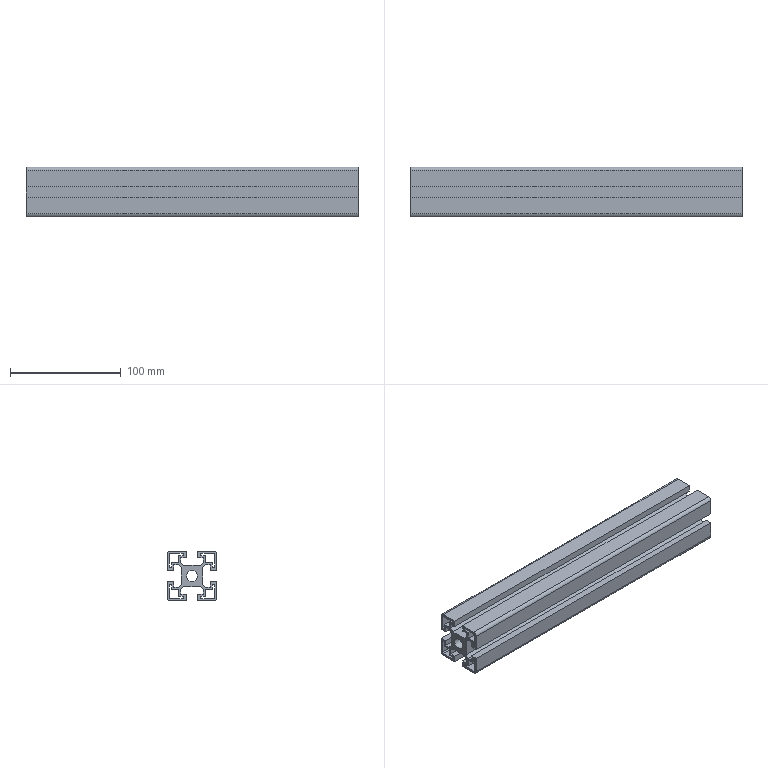Part | STEP file | 1_6 | 1 solid | 87 faces | box 300 x 45 x 45 mm | volume 245323 mm3 | plane 78 | cylinder 9 | commonest cylinder face diameters 2 x4 6 x4 10 x1